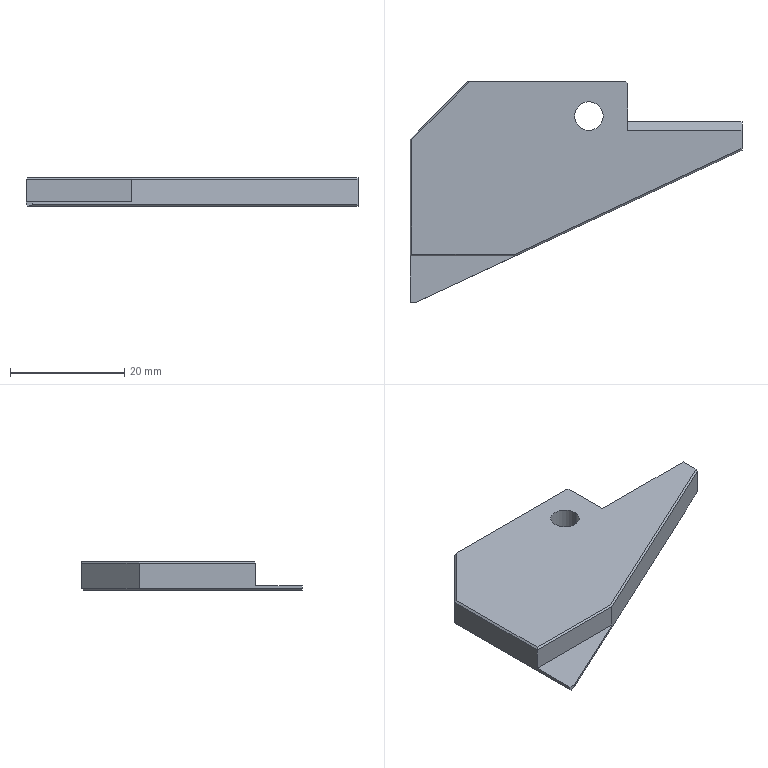Part | NX | 1 solid | 25 faces | box 58 x 38.5 x 5 mm | volume 5955 mm3 | plane 23 | cylinder 2 | commonest cylinder face diameters 5 x2
STEP:
#1=CARTESIAN_POINT('',(-132.,249.5,-29.5));
#2=VERTEX_POINT('',#1);
#3=CARTESIAN_POINT('',(-142.,239.5,-29.5));
#4=VERTEX_POINT('',#3);
#5=CARTESIAN_POINT('',(-137.,244.5,-29.5));
#6=DIRECTION('',(-0.7071,-0.7071,0.));
#7=VECTOR('',#6,1000.);
#8=LINE('',#5,#7);
#9=EDGE_CURVE('',#2,#4,#8,.T.);
#10=ORIENTED_EDGE('',*,*,#9,.F.);
#11=CARTESIAN_POINT('',(-131.876,249.2,-29.8));
#12=VERTEX_POINT('',#11);
#13=CARTESIAN_POINT('',(-130.561,246.027,-32.973));
#14=DIRECTION('',(-0.2811,0.6786,0.6786));
#15=VECTOR('',#14,1000.);
#16=LINE('',#13,#15);
#17=EDGE_CURVE('',#12,#2,#16,.T.);
#18=ORIENTED_EDGE('',*,*,#17,.F.);
#19=CARTESIAN_POINT('',(-141.7,239.376,-29.8));
#20=VERTEX_POINT('',#19);
#21=CARTESIAN_POINT('',(-136.788,244.288,-29.8));
#22=DIRECTION('',(-0.7071,-0.7071,0.));
#23=VECTOR('',#22,1000.);
#24=LINE('',#21,#23);
#25=EDGE_CURVE('',#12,#20,#24,.T.);
#26=ORIENTED_EDGE('',*,*,#25,.T.);
#27=CARTESIAN_POINT('',(-142.5,239.707,-29.));
#28=DIRECTION('',(0.6786,-0.2811,-0.6786));
#29=VECTOR('',#28,1000.);
#30=LINE('',#27,#29);
#31=EDGE_CURVE('',#4,#20,#30,.T.);
#32=ORIENTED_EDGE('',*,*,#31,.F.);
#33=EDGE_LOOP('',(#10,#18,#26,#32));
#34=FACE_BOUND('',#33,.T.);
#35=CARTESIAN_POINT('',(-136.894,244.394,-29.65));
#36=DIRECTION('',(-0.5,0.5,-0.7071));
#37=DIRECTION('',(-0.8165,0.,0.5774));
#38=AXIS2_PLACEMENT_3D('',#35,#36,#37);
#39=PLANE('',#38);
#40=ADVANCED_FACE('',(#34),#39,.T.);
#41=CARTESIAN_POINT('',(-142.,211.,-29.));
#42=VERTEX_POINT('',#41);
#43=CARTESIAN_POINT('',(-140.892,211.,-29.));
#44=VERTEX_POINT('',#43);
#45=CARTESIAN_POINT('',(-132.501,211.,-29.));
#46=DIRECTION('',(1.,0.,0.));
#47=VECTOR('',#46,1000.);
#48=LINE('',#45,#47);
#49=EDGE_CURVE('',#42,#44,#48,.T.);
#50=ORIENTED_EDGE('',*,*,#49,.F.);
#51=CARTESIAN_POINT('',(-142.,211.,-29.5));
#52=VERTEX_POINT('',#51);
#53=CARTESIAN_POINT('',(-142.,211.,-29.));
#54=DIRECTION('',(0.,0.,1.));
#55=VECTOR('',#54,1000.);
#56=LINE('',#53,#55);
#57=EDGE_CURVE('',#52,#42,#56,.T.);
#58=ORIENTED_EDGE('',*,*,#57,.F.);
#59=CARTESIAN_POINT('',(-141.7,211.,-29.8));
#60=VERTEX_POINT('',#59);
#61=CARTESIAN_POINT('',(-142.5,211.,-29.));
#62=DIRECTION('',(-0.7071,0.,0.7071));
#63=VECTOR('',#62,1000.);
#64=LINE('',#61,#63);
#65=EDGE_CURVE('',#60,#52,#64,.T.);
#66=ORIENTED_EDGE('',*,*,#65,.F.);
#67=CARTESIAN_POINT('',(-141.602,211.,-29.8));
#68=VERTEX_POINT('',#67);
#69=CARTESIAN_POINT('',(-132.501,211.,-29.8));
#70=DIRECTION('',(-1.,0.,0.));
#71=VECTOR('',#70,1000.);
#72=LINE('',#69,#71);
#73=EDGE_CURVE('',#68,#60,#72,.T.);
#74=ORIENTED_EDGE('',*,*,#73,.F.);
#75=CARTESIAN_POINT('',(-140.892,211.,-29.5));
#76=VERTEX_POINT('',#75);
#77=CARTESIAN_POINT('',(-132.501,211.,-25.954));
#78=DIRECTION('',(-0.9211,0.,-0.3893));
#79=VECTOR('',#78,1000.);
#80=LINE('',#77,#79);
#81=EDGE_CURVE('',#76,#68,#80,.T.);
#82=ORIENTED_EDGE('',*,*,#81,.F.);
#83=CARTESIAN_POINT('',(-140.892,211.,-29.));
#84=DIRECTION('',(0.,0.,-1.));
#85=VECTOR('',#84,1000.);
#86=LINE('',#83,#85);
#87=EDGE_CURVE('',#44,#76,#86,.T.);
#88=ORIENTED_EDGE('',*,*,#87,.F.);
#89=EDGE_LOOP('',(#50,#58,#66,#74,#82,#88));
#90=FACE_BOUND('',#89,.T.);
#91=CARTESIAN_POINT('',(-152.,211.,-29.));
#92=DIRECTION('',(0.,-1.,0.));
#93=DIRECTION('',(-1.,0.,0.));
#94=AXIS2_PLACEMENT_3D('',#91,#92,#93);
#95=PLANE('',#94);
#96=ADVANCED_FACE('',(#90),#95,.T.);
#97=CARTESIAN_POINT('',(-142.,225.25,-29.5));
#98=DIRECTION('',(0.,1.,0.));
#99=VECTOR('',#98,1000.);
#100=LINE('',#97,#99);
#101=EDGE_CURVE('',#52,#4,#100,.T.);
#102=ORIENTED_EDGE('',*,*,#101,.F.);
#103=ORIENTED_EDGE('',*,*,#57,.T.);
#104=CARTESIAN_POINT('',(-142.,219.1,-29.));
#105=VERTEX_POINT('',#104);
#106=CARTESIAN_POINT('',(-142.,246.027,-29.));
#107=DIRECTION('',(0.,-1.,0.));
#108=VECTOR('',#107,1000.);
#109=LINE('',#106,#108);
#110=EDGE_CURVE('',#105,#42,#109,.T.);
#111=ORIENTED_EDGE('',*,*,#110,.F.);
#112=CARTESIAN_POINT('',(-142.,219.1,-25.1));
#113=VERTEX_POINT('',#112);
#114=CARTESIAN_POINT('',(-142.,219.1,-29.));
#115=DIRECTION('',(0.,0.,-1.));
#116=VECTOR('',#115,1000.);
#117=LINE('',#114,#116);
#118=EDGE_CURVE('',#113,#105,#117,.T.);
#119=ORIENTED_EDGE('',*,*,#118,.F.);
#120=CARTESIAN_POINT('',(-142.,239.5,-25.1));
#121=VERTEX_POINT('',#120);
#122=CARTESIAN_POINT('',(-142.,229.088,-25.1));
#123=DIRECTION('',(0.,-1.,0.));
#124=VECTOR('',#123,1000.);
#125=LINE('',#122,#124);
#126=EDGE_CURVE('',#121,#113,#125,.T.);
#127=ORIENTED_EDGE('',*,*,#126,.F.);
#128=CARTESIAN_POINT('',(-142.,239.5,-29.));
#129=DIRECTION('',(0.,0.,1.));
#130=VECTOR('',#129,1000.);
#131=LINE('',#128,#130);
#132=EDGE_CURVE('',#4,#121,#131,.T.);
#133=ORIENTED_EDGE('',*,*,#132,.F.);
#134=EDGE_LOOP('',(#102,#103,#111,#119,#127,#133));
#135=FACE_BOUND('',#134,.T.);
#136=CARTESIAN_POINT('',(-142.,249.5,-29.));
#137=DIRECTION('',(-1.,0.,0.));
#138=DIRECTION('',(0.,0.,1.));
#139=AXIS2_PLACEMENT_3D('',#136,#137,#138);
#140=PLANE('',#139);
#141=ADVANCED_FACE('',(#135),#140,.T.);
#142=CARTESIAN_POINT('',(-84.,242.5,-28.3));
#143=VERTEX_POINT('',#142);
#144=CARTESIAN_POINT('',(-84.,242.5,-26.3));
#145=VERTEX_POINT('',#144);
#146=CARTESIAN_POINT('',(-84.,242.5,-29.));
#147=DIRECTION('',(0.,0.,1.));
#148=VECTOR('',#147,1000.);
#149=LINE('',#146,#148);
#150=EDGE_CURVE('',#143,#145,#149,.T.);
#151=ORIENTED_EDGE('',*,*,#150,.T.);
#152=CARTESIAN_POINT('',(-84.,241.,-24.8));
#153=VERTEX_POINT('',#152);
#154=CARTESIAN_POINT('',(-84.,245.2,-29.));
#155=DIRECTION('',(0.,0.7071,-0.7071));
#156=VECTOR('',#155,1000.);
#157=LINE('',#154,#156);
#158=EDGE_CURVE('',#153,#145,#157,.T.);
#159=ORIENTED_EDGE('',*,*,#158,.F.);
#160=CARTESIAN_POINT('',(-84.,237.86,-24.8));
#161=VERTEX_POINT('',#160);
#162=CARTESIAN_POINT('',(-84.,246.027,-24.8));
#163=DIRECTION('',(0.,-1.,0.));
#164=VECTOR('',#163,1000.);
#165=LINE('',#162,#164);
#166=EDGE_CURVE('',#153,#161,#165,.T.);
#167=ORIENTED_EDGE('',*,*,#166,.T.);
#168=CARTESIAN_POINT('',(-84.,237.529,-25.1));
#169=VERTEX_POINT('',#168);
#170=CARTESIAN_POINT('',(-84.,246.027,-17.399));
#171=DIRECTION('',(0.,-0.741,-0.6715));
#172=VECTOR('',#171,1000.);
#173=LINE('',#170,#172);
#174=EDGE_CURVE('',#161,#169,#173,.T.);
#175=ORIENTED_EDGE('',*,*,#174,.T.);
#176=CARTESIAN_POINT('',(-84.,237.529,-29.5));
#177=VERTEX_POINT('',#176);
#178=CARTESIAN_POINT('',(-84.,237.529,-29.));
#179=DIRECTION('',(0.,0.,-1.));
#180=VECTOR('',#179,1000.);
#181=LINE('',#178,#180);
#182=EDGE_CURVE('',#169,#177,#181,.T.);
#183=ORIENTED_EDGE('',*,*,#182,.T.);
#184=CARTESIAN_POINT('',(-84.,237.86,-29.8));
#185=VERTEX_POINT('',#184);
#186=CARTESIAN_POINT('',(-84.,246.027,-37.201));
#187=DIRECTION('',(0.,-0.741,0.6715));
#188=VECTOR('',#187,1000.);
#189=LINE('',#186,#188);
#190=EDGE_CURVE('',#185,#177,#189,.T.);
#191=ORIENTED_EDGE('',*,*,#190,.F.);
#192=CARTESIAN_POINT('',(-84.,241.,-29.8));
#193=VERTEX_POINT('',#192);
#194=CARTESIAN_POINT('',(-84.,246.027,-29.8));
#195=DIRECTION('',(0.,1.,0.));
#196=VECTOR('',#195,1000.);
#197=LINE('',#194,#196);
#198=EDGE_CURVE('',#185,#193,#197,.T.);
#199=ORIENTED_EDGE('',*,*,#198,.T.);
#200=CARTESIAN_POINT('',(-84.,241.8,-29.));
#201=DIRECTION('',(0.,-0.7071,-0.7071));
#202=VECTOR('',#201,1000.);
#203=LINE('',#200,#202);
#204=EDGE_CURVE('',#143,#193,#203,.T.);
#205=ORIENTED_EDGE('',*,*,#204,.F.);
#206=EDGE_LOOP('',(#151,#159,#167,#175,#183,#191,#199,#205));
#207=FACE_BOUND('',#206,.T.);
#208=CARTESIAN_POINT('',(-84.,243.5,-29.));
#209=DIRECTION('',(1.,0.,0.));
#210=DIRECTION('',(0.,-1.,0.));
#211=AXIS2_PLACEMENT_3D('',#208,#209,#210);
#212=PLANE('',#211);
#213=ADVANCED_FACE('',(#207),#212,.T.);
#214=CARTESIAN_POINT('',(-132.,249.5,-25.1));
#215=VERTEX_POINT('',#214);
#216=CARTESIAN_POINT('',(-137.,244.5,-25.1));
#217=DIRECTION('',(0.7071,0.7071,0.));
#218=VECTOR('',#217,1000.);
#219=LINE('',#216,#218);
#220=EDGE_CURVE('',#121,#215,#219,.T.);
#221=ORIENTED_EDGE('',*,*,#220,.T.);
#222=CARTESIAN_POINT('',(-132.,249.5,-29.));
#223=DIRECTION('',(0.,0.,1.));
#224=VECTOR('',#223,1000.);
#225=LINE('',#222,#224);
#226=EDGE_CURVE('',#2,#215,#225,.T.);
#227=ORIENTED_EDGE('',*,*,#226,.F.);
#228=ORIENTED_EDGE('',*,*,#9,.T.);
#229=ORIENTED_EDGE('',*,*,#132,.T.);
#230=EDGE_LOOP('',(#221,#227,#228,#229));
#231=FACE_BOUND('',#230,.T.);
#232=CARTESIAN_POINT('',(-137.,244.5,-31.45));
#233=DIRECTION('',(0.7071,-0.7071,0.));
#234=DIRECTION('',(0.,0.,-1.));
#235=AXIS2_PLACEMENT_3D('',#232,#233,#234);
#236=PLANE('',#235);
#237=ADVANCED_FACE('',(#231),#236,.F.);
#238=ORIENTED_EDGE('',*,*,#220,.F.);
#239=CARTESIAN_POINT('',(-141.7,239.376,-24.8));
#240=VERTEX_POINT('',#239);
#241=CARTESIAN_POINT('',(-132.501,235.566,-15.601));
#242=DIRECTION('',(-0.6786,0.2811,-0.6786));
#243=VECTOR('',#242,1000.);
#244=LINE('',#241,#243);
#245=EDGE_CURVE('',#240,#121,#244,.T.);
#246=ORIENTED_EDGE('',*,*,#245,.F.);
#247=CARTESIAN_POINT('',(-131.576,249.5,-24.8));
#248=VERTEX_POINT('',#247);
#249=CARTESIAN_POINT('',(-136.788,244.288,-24.8));
#250=DIRECTION('',(0.7071,0.7071,0.));
#251=VECTOR('',#250,1000.);
#252=LINE('',#249,#251);
#253=EDGE_CURVE('',#240,#248,#252,.T.);
#254=ORIENTED_EDGE('',*,*,#253,.T.);
#255=CARTESIAN_POINT('',(-132.501,249.5,-25.455));
#256=DIRECTION('',(-0.8165,0.,-0.5774));
#257=VECTOR('',#256,1000.);
#258=LINE('',#255,#257);
#259=EDGE_CURVE('',#248,#215,#258,.T.);
#260=ORIENTED_EDGE('',*,*,#259,.T.);
#261=EDGE_LOOP('',(#238,#246,#254,#260));
#262=FACE_BOUND('',#261,.T.);
#263=CARTESIAN_POINT('',(-136.894,244.394,-24.95));
#264=DIRECTION('',(-0.5,0.5,0.7071));
#265=DIRECTION('',(0.7071,0.7071,0.));
#266=AXIS2_PLACEMENT_3D('',#263,#264,#265);
#267=PLANE('',#266);
#268=ADVANCED_FACE('',(#262),#267,.T.);
#269=CARTESIAN_POINT('',(-104.,241.,-29.8));
#270=VERTEX_POINT('',#269);
#271=CARTESIAN_POINT('',(-94.,241.,-29.8));
#272=DIRECTION('',(1.,0.,0.));
#273=VECTOR('',#272,1000.);
#274=LINE('',#271,#273);
#275=EDGE_CURVE('',#270,#193,#274,.T.);
#276=ORIENTED_EDGE('',*,*,#275,.T.);
#277=ORIENTED_EDGE('',*,*,#198,.F.);
#278=CARTESIAN_POINT('',(-132.501,215.244,-29.8));
#279=DIRECTION('',(-0.9063,-0.4226,0.));
#280=VECTOR('',#279,1000.);
#281=LINE('',#278,#280);
#282=EDGE_CURVE('',#185,#68,#281,.T.);
#283=ORIENTED_EDGE('',*,*,#282,.T.);
#284=ORIENTED_EDGE('',*,*,#73,.T.);
#285=CARTESIAN_POINT('',(-141.7,225.25,-29.8));
#286=DIRECTION('',(0.,1.,0.));
#287=VECTOR('',#286,1000.);
#288=LINE('',#285,#287);
#289=EDGE_CURVE('',#60,#20,#288,.T.);
#290=ORIENTED_EDGE('',*,*,#289,.T.);
#291=ORIENTED_EDGE('',*,*,#25,.F.);
#292=CARTESIAN_POINT('',(-104.,249.2,-29.8));
#293=VERTEX_POINT('',#292);
#294=CARTESIAN_POINT('',(-132.501,249.2,-29.8));
#295=DIRECTION('',(1.,0.,0.));
#296=VECTOR('',#295,1000.);
#297=LINE('',#294,#296);
#298=EDGE_CURVE('',#12,#293,#297,.T.);
#299=ORIENTED_EDGE('',*,*,#298,.T.);
#300=CARTESIAN_POINT('',(-104.,246.027,-29.8));
#301=DIRECTION('',(0.,-1.,0.));
#302=VECTOR('',#301,1000.);
#303=LINE('',#300,#302);
#304=EDGE_CURVE('',#293,#270,#303,.T.);
#305=ORIENTED_EDGE('',*,*,#304,.T.);
#306=EDGE_LOOP('',(#276,#277,#283,#284,#290,#291,#299,#305));
#307=FACE_BOUND('',#306,.T.);
#308=CARTESIAN_POINT('',(-113.247,243.5,-29.8));
#309=VERTEX_POINT('',#308);
#310=CARTESIAN_POINT('',(-108.247,243.5,-29.8));
#311=VERTEX_POINT('',#310);
#312=CARTESIAN_POINT('',(-110.747,243.5,-29.8));
#313=DIRECTION('',(0.,0.,-1.));
#314=DIRECTION('',(-1.,0.,0.));
#315=AXIS2_PLACEMENT_3D('',#312,#313,#314);
#316=CIRCLE('',#315,2.5);
#317=EDGE_CURVE('',#309,#311,#316,.T.);
#318=ORIENTED_EDGE('',*,*,#317,.F.);
#319=CARTESIAN_POINT('',(-110.747,243.5,-29.8));
#320=DIRECTION('',(0.,0.,-1.));
#321=DIRECTION('',(-1.,0.,0.));
#322=AXIS2_PLACEMENT_3D('',#319,#320,#321);
#323=CIRCLE('',#322,2.5);
#324=EDGE_CURVE('',#311,#309,#323,.T.);
#325=ORIENTED_EDGE('',*,*,#324,.F.);
#326=EDGE_LOOP('',(#318,#325));
#327=FACE_BOUND('',#326,.T.);
#328=CARTESIAN_POINT('',(-92.,237.5,-29.8));
#329=DIRECTION('',(0.,0.,1.));
#330=DIRECTION('',(1.,0.,0.));
#331=AXIS2_PLACEMENT_3D('',#328,#329,#330);
#332=PLANE('',#331);
#333=ADVANCED_FACE('',(#307,#327),#332,.F.);
#334=CARTESIAN_POINT('',(-104.3,249.5,-29.5));
#335=VERTEX_POINT('',#334);
#336=CARTESIAN_POINT('',(-100.827,246.027,-32.973));
#337=DIRECTION('',(-0.5774,0.5774,0.5774));
#338=VECTOR('',#337,1000.);
#339=LINE('',#336,#338);
#340=EDGE_CURVE('',#293,#335,#339,.T.);
#341=ORIENTED_EDGE('',*,*,#340,.F.);
#342=ORIENTED_EDGE('',*,*,#298,.F.);
#343=ORIENTED_EDGE('',*,*,#17,.T.);
#344=CARTESIAN_POINT('',(-132.501,249.5,-29.5));
#345=DIRECTION('',(1.,0.,0.));
#346=VECTOR('',#345,1000.);
#347=LINE('',#344,#346);
#348=EDGE_CURVE('',#2,#335,#347,.T.);
#349=ORIENTED_EDGE('',*,*,#348,.T.);
#350=EDGE_LOOP('',(#341,#342,#343,#349));
#351=FACE_BOUND('',#350,.T.);
#352=CARTESIAN_POINT('',(-119.5,249.35,-29.65));
#353=DIRECTION('',(0.,0.7071,-0.7071));
#354=DIRECTION('',(-1.,0.,0.));
#355=AXIS2_PLACEMENT_3D('',#352,#353,#354);
#356=PLANE('',#355);
#357=ADVANCED_FACE('',(#351),#356,.T.);
#358=ORIENTED_EDGE('',*,*,#282,.F.);
#359=ORIENTED_EDGE('',*,*,#190,.T.);
#360=CARTESIAN_POINT('',(-132.501,214.913,-29.5));
#361=DIRECTION('',(-0.9063,-0.4226,0.));
#362=VECTOR('',#361,1000.);
#363=LINE('',#360,#362);
#364=EDGE_CURVE('',#177,#76,#363,.T.);
#365=ORIENTED_EDGE('',*,*,#364,.T.);
#366=ORIENTED_EDGE('',*,*,#81,.T.);
#367=EDGE_LOOP('',(#358,#359,#365,#366));
#368=FACE_BOUND('',#367,.T.);
#369=CARTESIAN_POINT('',(-111.509,224.867,-29.65));
#370=DIRECTION('',(0.2988,-0.6409,-0.7071));
#371=DIRECTION('',(0.,-0.741,0.6715));
#372=AXIS2_PLACEMENT_3D('',#369,#370,#371);
#373=PLANE('',#372);
#374=ADVANCED_FACE('',(#368),#373,.T.);
#375=ORIENTED_EDGE('',*,*,#289,.F.);
#376=ORIENTED_EDGE('',*,*,#65,.T.);
#377=ORIENTED_EDGE('',*,*,#101,.T.);
#378=ORIENTED_EDGE('',*,*,#31,.T.);
#379=EDGE_LOOP('',(#375,#376,#377,#378));
#380=FACE_BOUND('',#379,.T.);
#381=CARTESIAN_POINT('',(-141.85,225.25,-29.65));
#382=DIRECTION('',(-0.7071,0.,-0.7071));
#383=DIRECTION('',(-0.7071,0.,0.7071));
#384=AXIS2_PLACEMENT_3D('',#381,#382,#383);
#385=PLANE('',#384);
#386=ADVANCED_FACE('',(#380),#385,.T.);
#387=CARTESIAN_POINT('',(-104.3,249.5,-24.8));
#388=VERTEX_POINT('',#387);
#389=CARTESIAN_POINT('',(-104.3,249.5,-27.15));
#390=DIRECTION('',(0.,0.,1.));
#391=VECTOR('',#390,1000.);
#392=LINE('',#389,#391);
#393=EDGE_CURVE('',#335,#388,#392,.T.);
#394=ORIENTED_EDGE('',*,*,#393,.F.);
#395=ORIENTED_EDGE('',*,*,#348,.F.);
#396=ORIENTED_EDGE('',*,*,#226,.T.);
#397=ORIENTED_EDGE('',*,*,#259,.F.);
#398=CARTESIAN_POINT('',(-132.501,249.5,-24.8));
#399=DIRECTION('',(-1.,0.,0.));
#400=VECTOR('',#399,1000.);
#401=LINE('',#398,#400);
#402=EDGE_CURVE('',#388,#248,#401,.T.);
#403=ORIENTED_EDGE('',*,*,#402,.F.);
#404=EDGE_LOOP('',(#394,#395,#396,#397,#403));
#405=FACE_BOUND('',#404,.T.);
#406=CARTESIAN_POINT('',(-117.,249.5,-29.));
#407=DIRECTION('',(0.,1.,0.));
#408=DIRECTION('',(0.,0.,-1.));
#409=AXIS2_PLACEMENT_3D('',#406,#407,#408);
#410=PLANE('',#409);
#411=ADVANCED_FACE('',(#405),#410,.T.);
#412=ORIENTED_EDGE('',*,*,#150,.F.);
#413=CARTESIAN_POINT('',(-104.,242.5,-28.3));
#414=VERTEX_POINT('',#413);
#415=CARTESIAN_POINT('',(-94.,242.5,-28.3));
#416=DIRECTION('',(1.,0.,0.));
#417=VECTOR('',#416,1000.);
#418=LINE('',#415,#417);
#419=EDGE_CURVE('',#414,#143,#418,.T.);
#420=ORIENTED_EDGE('',*,*,#419,.F.);
#421=CARTESIAN_POINT('',(-104.,242.5,-26.3));
#422=VERTEX_POINT('',#421);
#423=CARTESIAN_POINT('',(-104.,242.5,-29.));
#424=DIRECTION('',(0.,0.,1.));
#425=VECTOR('',#424,1000.);
#426=LINE('',#423,#425);
#427=EDGE_CURVE('',#414,#422,#426,.T.);
#428=ORIENTED_EDGE('',*,*,#427,.T.);
#429=CARTESIAN_POINT('',(-94.,242.5,-26.3));
#430=DIRECTION('',(-1.,0.,0.));
#431=VECTOR('',#430,1000.);
#432=LINE('',#429,#431);
#433=EDGE_CURVE('',#145,#422,#432,.T.);
#434=ORIENTED_EDGE('',*,*,#433,.F.);
#435=EDGE_LOOP('',(#412,#420,#428,#434));
#436=FACE_BOUND('',#435,.T.);
#437=CARTESIAN_POINT('',(-102.,242.5,-24.3));
#438=DIRECTION('',(0.,-1.,0.));
#439=DIRECTION('',(-1.,0.,0.));
#440=AXIS2_PLACEMENT_3D('',#437,#438,#439);
#441=PLANE('',#440);
#442=ADVANCED_FACE('',(#436),#441,.F.);
#443=CARTESIAN_POINT('',(-104.,249.2,-24.8));
#444=VERTEX_POINT('',#443);
#445=CARTESIAN_POINT('',(-104.,249.2,-27.15));
#446=DIRECTION('',(0.,0.,1.));
#447=VECTOR('',#446,1000.);
#448=LINE('',#445,#447);
#449=EDGE_CURVE('',#293,#444,#448,.T.);
#450=ORIENTED_EDGE('',*,*,#449,.T.);
#451=CARTESIAN_POINT('',(-104.,241.,-24.8));
#452=VERTEX_POINT('',#451);
#453=CARTESIAN_POINT('',(-104.,246.027,-24.8));
#454=DIRECTION('',(0.,1.,0.));
#455=VECTOR('',#454,1000.);
#456=LINE('',#453,#455);
#457=EDGE_CURVE('',#452,#444,#456,.T.);
#458=ORIENTED_EDGE('',*,*,#457,.F.);
#459=CARTESIAN_POINT('',(-104.,245.2,-29.));
#460=DIRECTION('',(0.,-0.7071,0.7071));
#461=VECTOR('',#460,1000.);
#462=LINE('',#459,#461);
#463=EDGE_CURVE('',#422,#452,#462,.T.);
#464=ORIENTED_EDGE('',*,*,#463,.F.);
#465=ORIENTED_EDGE('',*,*,#427,.F.);
#466=CARTESIAN_POINT('',(-104.,241.8,-29.));
#467=DIRECTION('',(0.,0.7071,0.7071));
#468=VECTOR('',#467,1000.);
#469=LINE('',#466,#468);
#470=EDGE_CURVE('',#270,#414,#469,.T.);
#471=ORIENTED_EDGE('',*,*,#470,.F.);
#472=ORIENTED_EDGE('',*,*,#304,.F.);
#473=EDGE_LOOP('',(#450,#458,#464,#465,#471,#472));
#474=FACE_BOUND('',#473,.T.);
#475=CARTESIAN_POINT('',(-104.,261.676,-24.3));
#476=DIRECTION('',(-1.,0.,0.));
#477=DIRECTION('',(0.,0.,1.));
#478=AXIS2_PLACEMENT_3D('',#475,#476,#477);
#479=PLANE('',#478);
#480=ADVANCED_FACE('',(#474),#479,.F.);
#481=ORIENTED_EDGE('',*,*,#275,.F.);
#482=ORIENTED_EDGE('',*,*,#470,.T.);
#483=ORIENTED_EDGE('',*,*,#419,.T.);
#484=ORIENTED_EDGE('',*,*,#204,.T.);
#485=EDGE_LOOP('',(#481,#482,#483,#484));
#486=FACE_BOUND('',#485,.T.);
#487=CARTESIAN_POINT('',(-94.,241.75,-29.05));
#488=DIRECTION('',(0.,0.7071,-0.7071));
#489=DIRECTION('',(-1.,0.,0.));
#490=AXIS2_PLACEMENT_3D('',#487,#488,#489);
#491=PLANE('',#490);
#492=ADVANCED_FACE('',(#486),#491,.T.);
#493=ORIENTED_EDGE('',*,*,#449,.F.);
#494=ORIENTED_EDGE('',*,*,#340,.T.);
#495=ORIENTED_EDGE('',*,*,#393,.T.);
#496=CARTESIAN_POINT('',(-100.827,246.027,-24.8));
#497=DIRECTION('',(-0.7071,0.7071,0.));
#498=VECTOR('',#497,1000.);
#499=LINE('',#496,#498);
#500=EDGE_CURVE('',#444,#388,#499,.T.);
#501=ORIENTED_EDGE('',*,*,#500,.F.);
#502=EDGE_LOOP('',(#493,#494,#495,#501));
#503=FACE_BOUND('',#502,.T.);
#504=CARTESIAN_POINT('',(-104.15,249.35,-27.15));
#505=DIRECTION('',(0.7071,0.7071,0.));
#506=DIRECTION('',(0.,0.,-1.));
#507=AXIS2_PLACEMENT_3D('',#504,#505,#506);
#508=PLANE('',#507);
#509=ADVANCED_FACE('',(#503),#508,.T.);
#510=ORIENTED_EDGE('',*,*,#317,.T.);
#511=CARTESIAN_POINT('',(-108.247,243.5,-24.8));
#512=VERTEX_POINT('',#511);
#513=CARTESIAN_POINT('',(-108.247,243.5,-29.));
#514=DIRECTION('',(0.,0.,-1.));
#515=VECTOR('',#514,1000.);
#516=LINE('',#513,#515);
#517=EDGE_CURVE('',#512,#311,#516,.T.);
#518=ORIENTED_EDGE('',*,*,#517,.F.);
#519=CARTESIAN_POINT('',(-113.247,243.5,-24.8));
#520=VERTEX_POINT('',#519);
#521=CARTESIAN_POINT('',(-110.747,243.5,-24.8));
#522=DIRECTION('',(0.,0.,-1.));
#523=DIRECTION('',(-1.,0.,0.));
#524=AXIS2_PLACEMENT_3D('',#521,#522,#523);
#525=CIRCLE('',#524,2.5);
#526=EDGE_CURVE('',#520,#512,#525,.T.);
#527=ORIENTED_EDGE('',*,*,#526,.F.);
#528=CARTESIAN_POINT('',(-113.247,243.5,-29.));
#529=DIRECTION('',(0.,0.,-1.));
#530=VECTOR('',#529,1000.);
#531=LINE('',#528,#530);
#532=EDGE_CURVE('',#520,#309,#531,.T.);
#533=ORIENTED_EDGE('',*,*,#532,.T.);
#534=EDGE_LOOP('',(#510,#518,#527,#533));
#535=FACE_BOUND('',#534,.T.);
#536=CARTESIAN_POINT('',(-110.747,243.5,-29.));
#537=DIRECTION('',(0.,0.,-1.));
#538=DIRECTION('',(-1.,0.,0.));
#539=AXIS2_PLACEMENT_3D('',#536,#537,#538);
#540=CYLINDRICAL_SURFACE('',#539,2.5);
#541=ADVANCED_FACE('',(#535),#540,.F.);
#542=CARTESIAN_POINT('',(-141.7,219.4,-24.8));
#543=VERTEX_POINT('',#542);
#544=CARTESIAN_POINT('',(-123.588,219.4,-24.8));
#545=VERTEX_POINT('',#544);
#546=CARTESIAN_POINT('',(-132.966,219.4,-24.8));
#547=DIRECTION('',(1.,0.,0.));
#548=VECTOR('',#547,1000.);
#549=LINE('',#546,#548);
#550=EDGE_CURVE('',#543,#545,#549,.T.);
#551=ORIENTED_EDGE('',*,*,#550,.F.);
#552=CARTESIAN_POINT('',(-115.073,246.027,1.827));
#553=DIRECTION('',(-0.5774,-0.5774,-0.5774));
#554=VECTOR('',#553,1000.);
#555=LINE('',#552,#554);
#556=EDGE_CURVE('',#543,#113,#555,.T.);
#557=ORIENTED_EDGE('',*,*,#556,.T.);
#558=CARTESIAN_POINT('',(-123.522,219.1,-25.1));
#559=VERTEX_POINT('',#558);
#560=CARTESIAN_POINT('',(-132.966,219.1,-25.1));
#561=DIRECTION('',(1.,0.,0.));
#562=VECTOR('',#561,1000.);
#563=LINE('',#560,#562);
#564=EDGE_CURVE('',#113,#559,#563,.T.);
#565=ORIENTED_EDGE('',*,*,#564,.T.);
#566=CARTESIAN_POINT('',(-129.491,246.027,1.827));
#567=DIRECTION('',(0.1549,-0.6986,-0.6986));
#568=VECTOR('',#567,1000.);
#569=LINE('',#566,#568);
#570=EDGE_CURVE('',#545,#559,#569,.T.);
#571=ORIENTED_EDGE('',*,*,#570,.F.);
#572=EDGE_LOOP('',(#551,#557,#565,#571));
#573=FACE_BOUND('',#572,.T.);
#574=CARTESIAN_POINT('',(-132.966,219.25,-24.95));
#575=DIRECTION('',(0.,-0.7071,0.7071));
#576=DIRECTION('',(-1.,0.,0.));
#577=AXIS2_PLACEMENT_3D('',#574,#575,#576);
#578=PLANE('',#577);
#579=ADVANCED_FACE('',(#573),#578,.T.);
#580=ORIENTED_EDGE('',*,*,#550,.T.);
#581=CARTESIAN_POINT('',(-103.888,228.587,-24.8));
#582=DIRECTION('',(-0.9063,-0.4226,0.));
#583=VECTOR('',#582,1000.);
#584=LINE('',#581,#583);
#585=EDGE_CURVE('',#161,#545,#584,.T.);
#586=ORIENTED_EDGE('',*,*,#585,.F.);
#587=ORIENTED_EDGE('',*,*,#166,.F.);
#588=CARTESIAN_POINT('',(-94.,241.,-24.8));
#589=DIRECTION('',(-1.,0.,0.));
#590=VECTOR('',#589,1000.);
#591=LINE('',#588,#590);
#592=EDGE_CURVE('',#153,#452,#591,.T.);
#593=ORIENTED_EDGE('',*,*,#592,.T.);
#594=ORIENTED_EDGE('',*,*,#457,.T.);
#595=ORIENTED_EDGE('',*,*,#500,.T.);
#596=ORIENTED_EDGE('',*,*,#402,.T.);
#597=ORIENTED_EDGE('',*,*,#253,.F.);
#598=CARTESIAN_POINT('',(-141.7,229.088,-24.8));
#599=DIRECTION('',(0.,-1.,0.));
#600=VECTOR('',#599,1000.);
#601=LINE('',#598,#600);
#602=EDGE_CURVE('',#240,#543,#601,.T.);
#603=ORIENTED_EDGE('',*,*,#602,.T.);
#604=EDGE_LOOP('',(#580,#586,#587,#593,#594,#595,#596,#597,#603));
#605=FACE_BOUND('',#604,.T.);
#606=CARTESIAN_POINT('',(-110.747,243.5,-24.8));
#607=DIRECTION('',(0.,0.,-1.));
#608=DIRECTION('',(-1.,0.,0.));
#609=AXIS2_PLACEMENT_3D('',#606,#607,#608);
#610=CIRCLE('',#609,2.5);
#611=EDGE_CURVE('',#512,#520,#610,.T.);
#612=ORIENTED_EDGE('',*,*,#611,.T.);
#613=ORIENTED_EDGE('',*,*,#526,.T.);
#614=EDGE_LOOP('',(#612,#613));
#615=FACE_BOUND('',#614,.T.);
#616=CARTESIAN_POINT('',(-132.501,246.027,-24.8));
#617=DIRECTION('',(0.,0.,-1.));
#618=DIRECTION('',(0.,-1.,0.));
#619=AXIS2_PLACEMENT_3D('',#616,#617,#618);
#620=PLANE('',#619);
#621=ADVANCED_FACE('',(#605,#615),#620,.F.);
#622=ORIENTED_EDGE('',*,*,#182,.F.);
#623=CARTESIAN_POINT('',(-103.761,228.315,-25.1));
#624=DIRECTION('',(-0.9063,-0.4226,0.));
#625=VECTOR('',#624,1000.);
#626=LINE('',#623,#625);
#627=EDGE_CURVE('',#169,#559,#626,.T.);
#628=ORIENTED_EDGE('',*,*,#627,.T.);
#629=CARTESIAN_POINT('',(-123.522,219.1,-29.));
#630=VERTEX_POINT('',#629);
#631=CARTESIAN_POINT('',(-123.522,219.1,-29.));
#632=DIRECTION('',(0.,0.,-1.));
#633=VECTOR('',#632,1000.);
#634=LINE('',#631,#633);
#635=EDGE_CURVE('',#559,#630,#634,.T.);
#636=ORIENTED_EDGE('',*,*,#635,.T.);
#637=CARTESIAN_POINT('',(-132.501,214.913,-29.));
#638=DIRECTION('',(-0.9063,-0.4226,0.));
#639=VECTOR('',#638,1000.);
#640=LINE('',#637,#639);
#641=EDGE_CURVE('',#630,#44,#640,.T.);
#642=ORIENTED_EDGE('',*,*,#641,.T.);
#643=ORIENTED_EDGE('',*,*,#87,.T.);
#644=ORIENTED_EDGE('',*,*,#364,.F.);
#645=EDGE_LOOP('',(#622,#628,#636,#642,#643,#644));
#646=FACE_BOUND('',#645,.T.);
#647=CARTESIAN_POINT('',(-80.324,239.243,-28.51));
#648=DIRECTION('',(-0.4226,0.9063,0.));
#649=DIRECTION('',(0.,0.,1.));
#650=AXIS2_PLACEMENT_3D('',#647,#648,#649);
#651=PLANE('',#650);
#652=ADVANCED_FACE('',(#646),#651,.F.);
#653=ORIENTED_EDGE('',*,*,#635,.F.);
#654=ORIENTED_EDGE('',*,*,#564,.F.);
#655=ORIENTED_EDGE('',*,*,#118,.T.);
#656=CARTESIAN_POINT('',(-132.501,219.1,-29.));
#657=DIRECTION('',(-1.,0.,0.));
#658=VECTOR('',#657,1000.);
#659=LINE('',#656,#658);
#660=EDGE_CURVE('',#630,#105,#659,.T.);
#661=ORIENTED_EDGE('',*,*,#660,.F.);
#662=EDGE_LOOP('',(#653,#654,#655,#661));
#663=FACE_BOUND('',#662,.T.);
#664=CARTESIAN_POINT('',(-100.2,219.1,-28.2));
#665=DIRECTION('',(0.,1.,0.));
#666=DIRECTION('',(1.,0.,0.));
#667=AXIS2_PLACEMENT_3D('',#664,#665,#666);
#668=PLANE('',#667);
#669=ADVANCED_FACE('',(#663),#668,.F.);
#670=ORIENTED_EDGE('',*,*,#49,.T.);
#671=ORIENTED_EDGE('',*,*,#641,.F.);
#672=ORIENTED_EDGE('',*,*,#660,.T.);
#673=ORIENTED_EDGE('',*,*,#110,.T.);
#674=EDGE_LOOP('',(#670,#671,#672,#673));
#675=FACE_BOUND('',#674,.T.);
#676=CARTESIAN_POINT('',(-100.2,207.3,-29.));
#677=DIRECTION('',(0.,0.,-1.));
#678=DIRECTION('',(0.,-1.,0.));
#679=AXIS2_PLACEMENT_3D('',#676,#677,#678);
#680=PLANE('',#679);
#681=ADVANCED_FACE('',(#675),#680,.F.);
#682=ORIENTED_EDGE('',*,*,#592,.F.);
#683=ORIENTED_EDGE('',*,*,#158,.T.);
#684=ORIENTED_EDGE('',*,*,#433,.T.);
#685=ORIENTED_EDGE('',*,*,#463,.T.);
#686=EDGE_LOOP('',(#682,#683,#684,#685));
#687=FACE_BOUND('',#686,.T.);
#688=CARTESIAN_POINT('',(-94.,241.75,-25.55));
#689=DIRECTION('',(0.,0.7071,0.7071));
#690=DIRECTION('',(1.,0.,0.));
#691=AXIS2_PLACEMENT_3D('',#688,#689,#690);
#692=PLANE('',#691);
#693=ADVANCED_FACE('',(#687),#692,.T.);
#694=ORIENTED_EDGE('',*,*,#585,.T.);
#695=ORIENTED_EDGE('',*,*,#570,.T.);
#696=ORIENTED_EDGE('',*,*,#627,.F.);
#697=ORIENTED_EDGE('',*,*,#174,.F.);
#698=EDGE_LOOP('',(#694,#695,#696,#697));
#699=FACE_BOUND('',#698,.T.);
#700=CARTESIAN_POINT('',(-103.824,228.451,-24.95));
#701=DIRECTION('',(-0.2988,0.6409,-0.7071));
#702=DIRECTION('',(-0.9211,0.,0.3893));
#703=AXIS2_PLACEMENT_3D('',#700,#701,#702);
#704=PLANE('',#703);
#705=ADVANCED_FACE('',(#699),#704,.F.);
#706=ORIENTED_EDGE('',*,*,#602,.F.);
#707=ORIENTED_EDGE('',*,*,#245,.T.);
#708=ORIENTED_EDGE('',*,*,#126,.T.);
#709=ORIENTED_EDGE('',*,*,#556,.F.);
#710=EDGE_LOOP('',(#706,#707,#708,#709));
#711=FACE_BOUND('',#710,.T.);
#712=CARTESIAN_POINT('',(-141.85,229.088,-24.95));
#713=DIRECTION('',(-0.7071,0.,0.7071));
#714=DIRECTION('',(0.,1.,0.));
#715=AXIS2_PLACEMENT_3D('',#712,#713,#714);
#716=PLANE('',#715);
#717=ADVANCED_FACE('',(#711),#716,.T.);
#718=ORIENTED_EDGE('',*,*,#611,.F.);
#719=ORIENTED_EDGE('',*,*,#517,.T.);
#720=ORIENTED_EDGE('',*,*,#324,.T.);
#721=ORIENTED_EDGE('',*,*,#532,.F.);
#722=EDGE_LOOP('',(#718,#719,#720,#721));
#723=FACE_BOUND('',#722,.T.);
#724=CARTESIAN_POINT('',(-110.747,243.5,-29.));
#725=DIRECTION('',(0.,0.,-1.));
#726=DIRECTION('',(-1.,0.,0.));
#727=AXIS2_PLACEMENT_3D('',#724,#725,#726);
#728=CYLINDRICAL_SURFACE('',#727,2.5);
#729=ADVANCED_FACE('',(#723),#728,.F.);
#730=CLOSED_SHELL('',(#40,#96,#141,#213,#237,#268,#333,#357,#374,#386,#411,#442,#480,#492,#509,#541,#579,#621,#652,#669,#681,#693,#705,#717,#729));
#731=MANIFOLD_SOLID_BREP('',#730);
#732=(LENGTH_UNIT()NAMED_UNIT(*)SI_UNIT(.MILLI.,.METRE.));
#733=UNCERTAINTY_MEASURE_WITH_UNIT(LENGTH_MEASURE(0.00001),#732,'','');
#734=(NAMED_UNIT(*)PLANE_ANGLE_UNIT()SI_UNIT($,.RADIAN.));
#735=(NAMED_UNIT(*)SI_UNIT($,.STERADIAN.)SOLID_ANGLE_UNIT());
#736=(GEOMETRIC_REPRESENTATION_CONTEXT(3)GLOBAL_UNCERTAINTY_ASSIGNED_CONTEXT((#733))GLOBAL_UNIT_ASSIGNED_CONTEXT((#732,#734,#735))REPRESENTATION_CONTEXT('',''));
#737=ADVANCED_BREP_SHAPE_REPRESENTATION('',(#731),#736);